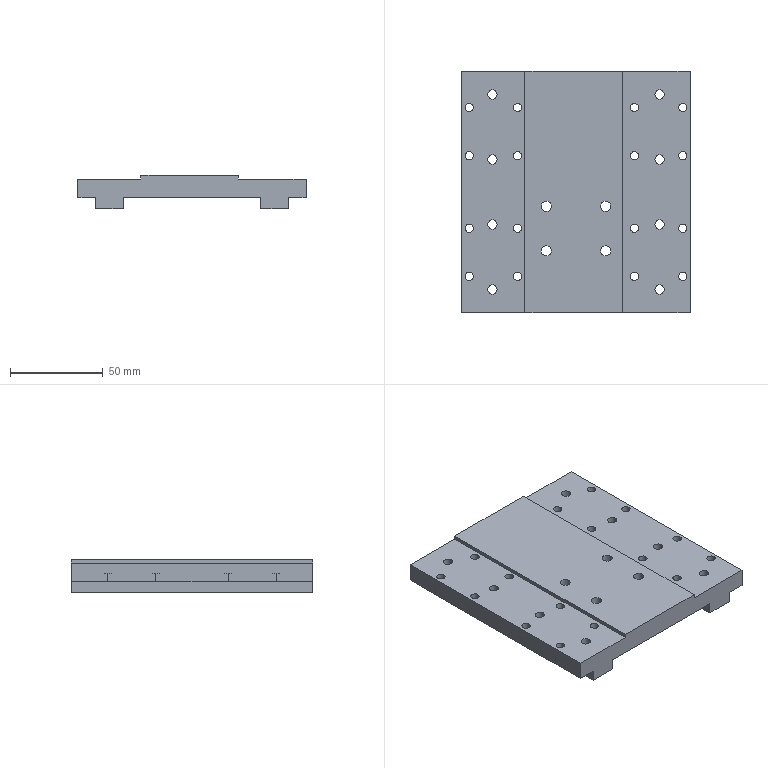NC program | NX | posted with a generic post | part box 123 x 130 x 18 mm
Lines 1850 to 2087 of 2087:
(ZLEVEL_PROFILE_COPY_1 , TOOL : D10JING)
N3650 T14 M6
N3652 G54
N3654 G17 G0 G90 X-65.25 Y-31.007 S9500 M3
N3656 G43 Z30. H14
N3658 Z-15.9
N3660 G94 G1 Y0. Z-17.525 F1000.
N3662 Y65. F1200.
N3664 G2 X-60.25 Y70. R5.
N3666 G1 X62.75
N3668 G2 X67.75 Y65. R5.
N3670 G1 Y-65.
N3672 G2 X62.75 Y-70. R5.
N3674 G1 X-60.25
N3676 G2 X-65.25 Y-65. R5.
N3678 G1 Y0.
N3680 Y65. Z-17.54
N3682 X-65.226 Y65.49
N3684 X-65.154 Y65.975
N3686 X-65.035 Y66.451
N3688 X-64.869 Y66.913 Z-17.541
N3690 X-64.66 Y67.357
N3692 X-64.407 Y67.778
N3694 X-64.115 Y68.172
N3696 X-63.786 Y68.536
N3698 X-63.422 Y68.865
N3700 X-63.028 Y69.157
N3702 X-62.607 Y69.41
N3704 X-62.163 Y69.619
N3706 X-61.701 Y69.785 Z-17.542
N3708 X-61.225 Y69.904
N3710 X-60.74 Y69.976
N3712 X-60.25 Y70.
N3714 X62.75 Z-17.571
N3716 X63.24 Y69.976
N3718 X63.725 Y69.904
N3720 X64.201 Y69.785
N3722 X64.663 Y69.619
N3724 X65.107 Y69.41
N3726 X65.528 Y69.157
N3728 X65.922 Y68.865
N3730 X66.286 Y68.536
N3732 X66.615 Y68.172 Z-17.572
N3734 X66.907 Y67.778
N3736 X67.16 Y67.357
N3738 X67.369 Y66.913
N3740 X67.535 Y66.451
N3742 X67.654 Y65.975
N3744 X67.726 Y65.49
N3746 X67.75 Y65.
N3748 Y-65. Z-17.603
N3750 X67.726 Y-65.49
N3752 X67.654 Y-65.975
N3754 X67.535 Y-66.451
N3756 X67.369 Y-66.913
N3758 X67.16 Y-67.357
N3760 X66.907 Y-67.778
N3762 X66.615 Y-68.172
N3764 X66.286 Y-68.536 Z-17.604
N3766 X65.922 Y-68.865
N3768 X65.528 Y-69.157
N3770 X65.107 Y-69.41
N3772 X64.663 Y-69.619
N3774 X64.201 Y-69.785
N3776 X63.725 Y-69.904
N3778 X63.24 Y-69.976
N3780 X62.75 Y-70.
N3782 X-60.25 Z-17.633
N3784 X-60.74 Y-69.976
N3786 X-61.225 Y-69.904
N3788 X-61.701 Y-69.785
N3790 X-62.163 Y-69.619 Z-17.634
N3792 X-62.607 Y-69.41
N3794 X-63.028 Y-69.157
N3796 X-63.422 Y-68.865
N3798 X-63.786 Y-68.536
N3800 X-64.115 Y-68.172
N3802 X-64.407 Y-67.778
N3804 X-64.66 Y-67.357
N3806 X-64.869 Y-66.913
N3808 X-65.035 Y-66.451 Z-17.635
N3810 X-65.154 Y-65.975
N3812 X-65.226 Y-65.49
N3814 X-65.25 Y-65.
N3816 Y0. Z-17.65
N3818 Y65. Z-17.665
N3820 X-65.226 Y65.49
N3822 X-65.154 Y65.975
N3824 X-65.035 Y66.451
N3826 X-64.869 Y66.913 Z-17.666
N3828 X-64.66 Y67.357
N3830 X-64.407 Y67.778
N3832 X-64.115 Y68.172
N3834 X-63.786 Y68.536
N3836 X-63.422 Y68.865
N3838 X-63.028 Y69.157
N3840 X-62.607 Y69.41
N3842 X-62.163 Y69.619
N3844 X-61.701 Y69.785 Z-17.667
N3846 X-61.225 Y69.904
N3848 X-60.74 Y69.976
N3850 X-60.25 Y70.
N3852 X62.75 Z-17.696
N3854 X63.24 Y69.976
N3856 X63.725 Y69.904
N3858 X64.201 Y69.785
N3860 X64.663 Y69.619
N3862 X65.107 Y69.41
N3864 X65.528 Y69.157
N3866 X65.922 Y68.865
N3868 X66.286 Y68.536
N3870 X66.615 Y68.172 Z-17.697
N3872 X66.907 Y67.778
N3874 X67.16 Y67.357
N3876 X67.369 Y66.913
N3878 X67.535 Y66.451
N3880 X67.654 Y65.975
N3882 X67.726 Y65.49
N3884 X67.75 Y65.
N3886 Y-65. Z-17.728
N3888 X67.726 Y-65.49
N3890 X67.654 Y-65.975
N3892 X67.535 Y-66.451
N3894 X67.369 Y-66.913
N3896 X67.16 Y-67.357
N3898 X66.907 Y-67.778
N3900 X66.615 Y-68.172
N3902 X66.286 Y-68.536 Z-17.729
N3904 X65.922 Y-68.865
N3906 X65.528 Y-69.157
N3908 X65.107 Y-69.41
N3910 X64.663 Y-69.619
N3912 X64.201 Y-69.785
N3914 X63.725 Y-69.904
N3916 X63.24 Y-69.976
N3918 X62.75 Y-70.
N3920 X-60.25 Z-17.758
N3922 X-60.74 Y-69.976
N3924 X-61.225 Y-69.904
N3926 X-61.701 Y-69.785
N3928 X-62.163 Y-69.619 Z-17.759
N3930 X-62.607 Y-69.41
N3932 X-63.028 Y-69.157
N3934 X-63.422 Y-68.865
N3936 X-63.786 Y-68.536
N3938 X-64.115 Y-68.172
N3940 X-64.407 Y-67.778
N3942 X-64.66 Y-67.357
N3944 X-64.869 Y-66.913
N3946 X-65.035 Y-66.451 Z-17.76
N3948 X-65.154 Y-65.975
N3950 X-65.226 Y-65.49
N3952 X-65.25 Y-65.
N3954 Y0. Z-17.775
N3956 Y65. Z-17.79
N3958 X-65.226 Y65.49
N3960 X-65.154 Y65.975
N3962 X-65.035 Y66.451
N3964 X-64.869 Y66.913 Z-17.791
N3966 X-64.66 Y67.357
N3968 X-64.407 Y67.778
N3970 X-64.115 Y68.172
N3972 X-63.786 Y68.536
N3974 X-63.422 Y68.865
N3976 X-63.028 Y69.157
N3978 X-62.607 Y69.41
N3980 X-62.163 Y69.619
N3982 X-61.701 Y69.785 Z-17.792
N3984 X-61.225 Y69.904
N3986 X-60.74 Y69.976
N3988 X-60.25 Y70.
N3990 X62.75 Z-17.821
N3992 X63.24 Y69.976
N3994 X63.725 Y69.904
N3996 X64.201 Y69.785
N3998 X64.663 Y69.619
N4000 X65.107 Y69.41
N4002 X65.528 Y69.157
N4004 X65.922 Y68.865
N4006 X66.286 Y68.536
N4008 X66.615 Y68.172 Z-17.822
N4010 X66.907 Y67.778
N4012 X67.16 Y67.357
N4014 X67.369 Y66.913
N4016 X67.535 Y66.451
N4018 X67.654 Y65.975
N4020 X67.726 Y65.49
N4022 X67.75 Y65.
N4024 Y-65. Z-17.853
N4026 X67.726 Y-65.49
N4028 X67.654 Y-65.975
N4030 X67.535 Y-66.451
N4032 X67.369 Y-66.913
N4034 X67.16 Y-67.357
N4036 X66.907 Y-67.778
N4038 X66.615 Y-68.172
N4040 X66.286 Y-68.536 Z-17.854
N4042 X65.922 Y-68.865
N4044 X65.528 Y-69.157
N4046 X65.107 Y-69.41
N4048 X64.663 Y-69.619
N4050 X64.201 Y-69.785
N4052 X63.725 Y-69.904
N4054 X63.24 Y-69.976
N4056 X62.75 Y-70.
N4058 X-60.25 Z-17.883
N4060 X-60.74 Y-69.976
N4062 X-61.225 Y-69.904
N4064 X-61.701 Y-69.785
N4066 X-62.163 Y-69.619 Z-17.884
N4068 X-62.607 Y-69.41
N4070 X-63.028 Y-69.157
N4072 X-63.422 Y-68.865
N4074 X-63.786 Y-68.536
N4076 X-64.115 Y-68.172
N4078 X-64.407 Y-67.778
N4080 X-64.66 Y-67.357
N4082 X-64.869 Y-66.913
N4084 X-65.035 Y-66.451 Z-17.885
N4086 X-65.154 Y-65.975
N4088 X-65.226 Y-65.49
N4090 X-65.25 Y-65.
N4092 Y0. Z-17.9
N4094 Y65.
N4096 G2 X-60.25 Y70. R5.
N4098 G1 X62.75
N4100 G2 X67.75 Y65. R5.
N4102 G1 Y-65.
N4104 G2 X62.75 Y-70. R5.
N4106 G1 X-60.25
N4108 G2 X-65.25 Y-65. R5.
N4110 G1 Y0.
N4112 Z-16.4
N4114 G0 Z30.
N4116 M5
N4118 M2